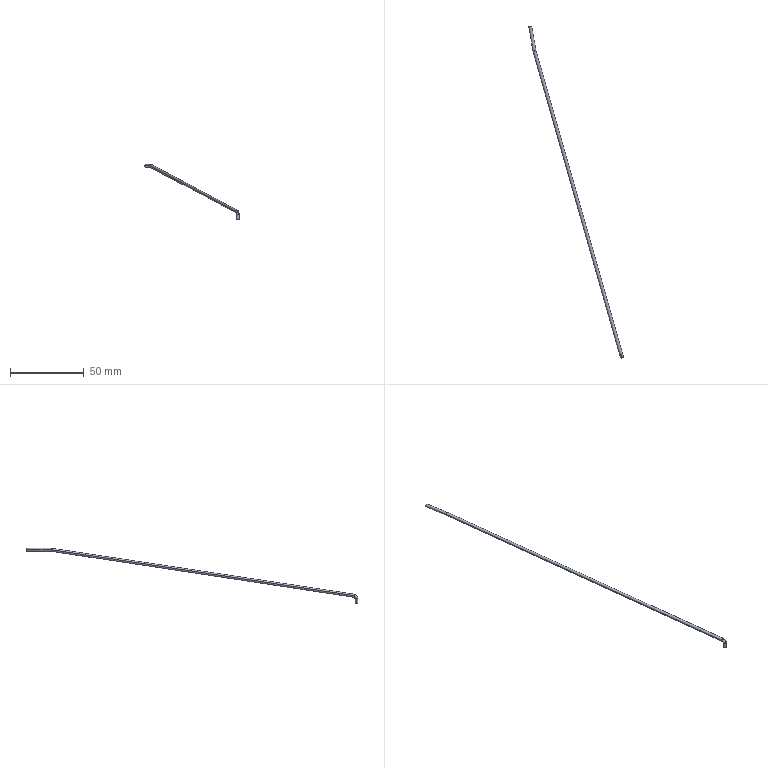Part | STEP file | rear_spoke3 | 1 solid | 10 faces | box 63.794 x 224.344 x 37.5 mm | volume 749.298 mm3 | cylinder 6 | torus 2 | plane 2 | commonest cylinder face diameters 2 x6
STEP:
#1=CARTESIAN_POINT('',(0.,0.,0.));
#2=DIRECTION('',(0.,0.,1.));
#3=DIRECTION('',(1.,0.,0.));
#4=AXIS2_PLACEMENT_3D('',#1,#2,#3);
#5=CARTESIAN_POINT('',(19.506,20.506,0.4406));
#6=VERTEX_POINT('',#5);
#7=CARTESIAN_POINT('',(20.781,19.545,0.4406));
#8=VERTEX_POINT('',#7);
#9=CARTESIAN_POINT('',(20.506,20.506,0.4406));
#10=DIRECTION('',(0.,0.,1.));
#11=DIRECTION('',(1.,0.,0.));
#12=AXIS2_PLACEMENT_3D('',#9,#10,#11);
#13=CIRCLE('',#12,1.);
#14=CARTESIAN_POINT('',(19.957,22.429,0.4406));
#15=DIRECTION('',(-0.9615,-0.2746,0.));
#16=DIRECTION('',(0.2746,-0.9615,0.));
#17=AXIS2_PLACEMENT_3D('',#14,#15,#16);
#18=TOROIDAL_SURFACE('',#17,2.,1.);
#19=CARTESIAN_POINT('',(0.,1.849));
#20=CARTESIAN_POINT('',(0.,1.821));
#21=CARTESIAN_POINT('',(0.,1.765));
#22=CARTESIAN_POINT('',(0.,1.681));
#23=CARTESIAN_POINT('',(0.,1.597));
#24=CARTESIAN_POINT('',(0.,1.513));
#25=CARTESIAN_POINT('',(0.,1.429));
#26=CARTESIAN_POINT('',(0.,1.345));
#27=CARTESIAN_POINT('',(0.,1.261));
#28=CARTESIAN_POINT('',(0.,1.177));
#29=CARTESIAN_POINT('',(0.,1.093));
#30=CARTESIAN_POINT('',(0.,1.009));
#31=CARTESIAN_POINT('',(0.,0.9245));
#32=CARTESIAN_POINT('',(0.,0.8405));
#33=CARTESIAN_POINT('',(0.,0.7564));
#34=CARTESIAN_POINT('',(0.,0.6724));
#35=CARTESIAN_POINT('',(0.,0.5883));
#36=CARTESIAN_POINT('',(0.,0.5043));
#37=CARTESIAN_POINT('',(0.,0.4202));
#38=CARTESIAN_POINT('',(0.,0.3362));
#39=CARTESIAN_POINT('',(0.,0.2521));
#40=CARTESIAN_POINT('',(0.,0.1681));
#41=CARTESIAN_POINT('',(0.,0.08405));
#42=CARTESIAN_POINT('',(0.,0.02802));
#43=CARTESIAN_POINT('',(0.,0.));
#44=B_SPLINE_CURVE_WITH_KNOTS('',3,(#19,#20,#21,#22,#23,#24,#25,#26,#27,#28,#29,#30,#31,#32,#33,#34,#35,#36,#37,#38,#39,#40,#41,#42,#43),.UNSPECIFIED.,.F.,.F.,(4,1,1,1,1,1,1,1,1,1,1,1,1,1,1,1,1,1,1,1,1,1,4),(3.142,3.226,3.31,3.394,3.478,3.562,3.646,3.73,3.814,3.898,3.982,4.066,4.15,4.234,4.318,4.402,4.486,4.57,4.654,4.738,4.823,4.907,4.991),.QUASI_UNIFORM_KNOTS.);
#45=(GEOMETRIC_REPRESENTATION_CONTEXT(2)PARAMETRIC_REPRESENTATION_CONTEXT()REPRESENTATION_CONTEXT('',''));
#46=DEFINITIONAL_REPRESENTATION('',(#44),#45);
#47=PCURVE('',#18,#46);
#48=CARTESIAN_POINT('',(20.506,20.506,-3.));
#49=DIRECTION('',(0.,0.,1.));
#50=DIRECTION('',(1.,0.,0.));
#51=AXIS2_PLACEMENT_3D('',#48,#49,#50);
#52=CYLINDRICAL_SURFACE('',#51,1.);
#53=CARTESIAN_POINT('',(0.,3.441));
#54=DIRECTION('',(1.,0.));
#55=VECTOR('',#54,1.);
#56=LINE('',#53,#55);
#57=(GEOMETRIC_REPRESENTATION_CONTEXT(2)PARAMETRIC_REPRESENTATION_CONTEXT()REPRESENTATION_CONTEXT('',''));
#58=DEFINITIONAL_REPRESENTATION('',(#56),#57);
#59=PCURVE('',#52,#58);
#60=SURFACE_CURVE('',#13,(#47,#59),.PCURVE_S1.);
#61=EDGE_CURVE('',#6,#8,#60,.T.);
#62=ORIENTED_EDGE('',*,*,#61,.T.);
#63=CARTESIAN_POINT('',(20.076,22.013,3.409));
#64=VERTEX_POINT('',#63);
#65=CARTESIAN_POINT('',(19.957,22.429,0.4406));
#66=DIRECTION('',(-0.9615,-0.2746,0.));
#67=DIRECTION('',(0.2746,-0.9615,0.));
#68=AXIS2_PLACEMENT_3D('',#65,#66,#67);
#69=CIRCLE('',#68,3.);
#70=CARTESIAN_POINT('',(0.,0.));
#71=DIRECTION('',(1.,0.));
#72=VECTOR('',#71,1.);
#73=LINE('',#70,#72);
#74=(GEOMETRIC_REPRESENTATION_CONTEXT(2)PARAMETRIC_REPRESENTATION_CONTEXT()REPRESENTATION_CONTEXT('',''));
#75=DEFINITIONAL_REPRESENTATION('',(#73),#74);
#76=PCURVE('',#18,#75);
#77=CARTESIAN_POINT('',(19.957,22.429,0.4406));
#78=DIRECTION('',(-0.9615,-0.2746,0.));
#79=DIRECTION('',(0.2746,-0.9615,0.));
#80=AXIS2_PLACEMENT_3D('',#77,#78,#79);
#81=TOROIDAL_SURFACE('',#80,2.,1.);
#82=CARTESIAN_POINT('',(0.,6.283));
#83=DIRECTION('',(1.,0.));
#84=VECTOR('',#83,1.);
#85=LINE('',#82,#84);
#86=(GEOMETRIC_REPRESENTATION_CONTEXT(2)PARAMETRIC_REPRESENTATION_CONTEXT()REPRESENTATION_CONTEXT('',''));
#87=DEFINITIONAL_REPRESENTATION('',(#85),#86);
#88=PCURVE('',#81,#87);
#89=SURFACE_CURVE('',#69,(#76,#88),.PCURVE_S1.);
#90=EDGE_CURVE('',#8,#64,#89,.T.);
#91=ORIENTED_EDGE('',*,*,#90,.T.);
#92=CARTESIAN_POINT('',(19.075,21.877,2.42));
#93=VERTEX_POINT('',#92);
#94=CARTESIAN_POINT('',(20.036,22.152,2.42));
#95=DIRECTION('',(-0.2718,0.9515,0.1444));
#96=DIRECTION('',(0.9355,0.226,0.2718));
#97=AXIS2_PLACEMENT_3D('',#94,#95,#96);
#98=CIRCLE('',#97,1.);
#99=CARTESIAN_POINT('',(1.426,4.991));
#100=DIRECTION('',(0.,-1.));
#101=VECTOR('',#100,1.);
#102=LINE('',#99,#101);
#103=(GEOMETRIC_REPRESENTATION_CONTEXT(2)PARAMETRIC_REPRESENTATION_CONTEXT()REPRESENTATION_CONTEXT('',''));
#104=DEFINITIONAL_REPRESENTATION('',(#102),#103);
#105=PCURVE('',#18,#104);
#106=CARTESIAN_POINT('',(20.036,22.152,2.42));
#107=DIRECTION('',(-0.2718,0.9515,0.1444));
#108=DIRECTION('',(-0.9615,-0.2746,0.));
#109=AXIS2_PLACEMENT_3D('',#106,#107,#108);
#110=CYLINDRICAL_SURFACE('',#109,1.);
#111=CARTESIAN_POINT('',(-3.42,0.));
#112=DIRECTION('',(1.,0.));
#113=VECTOR('',#112,1.);
#114=LINE('',#111,#113);
#115=(GEOMETRIC_REPRESENTATION_CONTEXT(2)PARAMETRIC_REPRESENTATION_CONTEXT()REPRESENTATION_CONTEXT('',''));
#116=DEFINITIONAL_REPRESENTATION('',(#114),#115);
#117=PCURVE('',#110,#116);
#118=SURFACE_CURVE('',#98,(#105,#117),.PCURVE_S1.);
#119=EDGE_CURVE('',#93,#64,#118,.T.);
#120=ORIENTED_EDGE('',*,*,#119,.F.);
#121=CARTESIAN_POINT('',(19.996,22.29,1.43));
#122=VERTEX_POINT('',#121);
#123=CARTESIAN_POINT('',(20.036,22.152,2.42));
#124=DIRECTION('',(-0.2718,0.9515,0.1444));
#125=DIRECTION('',(0.9355,0.226,0.2718));
#126=AXIS2_PLACEMENT_3D('',#123,#124,#125);
#127=CIRCLE('',#126,1.);
#128=CARTESIAN_POINT('',(1.426,4.991));
#129=DIRECTION('',(0.,-1.));
#130=VECTOR('',#129,1.);
#131=LINE('',#128,#130);
#132=(GEOMETRIC_REPRESENTATION_CONTEXT(2)PARAMETRIC_REPRESENTATION_CONTEXT()REPRESENTATION_CONTEXT('',''));
#133=DEFINITIONAL_REPRESENTATION('',(#131),#132);
#134=PCURVE('',#18,#133);
#135=CARTESIAN_POINT('',(20.036,22.152,2.42));
#136=DIRECTION('',(-0.2718,0.9515,0.1444));
#137=DIRECTION('',(-0.9615,-0.2746,0.));
#138=AXIS2_PLACEMENT_3D('',#135,#136,#137);
#139=CYLINDRICAL_SURFACE('',#138,1.);
#140=CARTESIAN_POINT('',(2.863,0.));
#141=DIRECTION('',(1.,0.));
#142=VECTOR('',#141,1.);
#143=LINE('',#140,#142);
#144=(GEOMETRIC_REPRESENTATION_CONTEXT(2)PARAMETRIC_REPRESENTATION_CONTEXT()REPRESENTATION_CONTEXT('',''));
#145=DEFINITIONAL_REPRESENTATION('',(#143),#144);
#146=PCURVE('',#139,#145);
#147=SURFACE_CURVE('',#127,(#134,#146),.PCURVE_S1.);
#148=EDGE_CURVE('',#122,#93,#147,.T.);
#149=ORIENTED_EDGE('',*,*,#148,.F.);
#150=CARTESIAN_POINT('',(20.231,21.468,0.4406));
#151=VERTEX_POINT('',#150);
#152=CARTESIAN_POINT('',(19.957,22.429,0.4406));
#153=DIRECTION('',(-0.9615,-0.2746,0.));
#154=DIRECTION('',(0.2746,-0.9615,0.));
#155=AXIS2_PLACEMENT_3D('',#152,#153,#154);
#156=CIRCLE('',#155,1.);
#157=CARTESIAN_POINT('',(0.,3.142));
#158=DIRECTION('',(1.,0.));
#159=VECTOR('',#158,1.);
#160=LINE('',#157,#159);
#161=(GEOMETRIC_REPRESENTATION_CONTEXT(2)PARAMETRIC_REPRESENTATION_CONTEXT()REPRESENTATION_CONTEXT('',''));
#162=DEFINITIONAL_REPRESENTATION('',(#160),#161);
#163=PCURVE('',#18,#162);
#164=CARTESIAN_POINT('',(0.,3.142));
#165=DIRECTION('',(1.,0.));
#166=VECTOR('',#165,1.);
#167=LINE('',#164,#166);
#168=(GEOMETRIC_REPRESENTATION_CONTEXT(2)PARAMETRIC_REPRESENTATION_CONTEXT()REPRESENTATION_CONTEXT('',''));
#169=DEFINITIONAL_REPRESENTATION('',(#167),#168);
#170=PCURVE('',#81,#169);
#171=SURFACE_CURVE('',#156,(#163,#170),.PCURVE_S1.);
#172=EDGE_CURVE('',#151,#122,#171,.T.);
#173=ORIENTED_EDGE('',*,*,#172,.F.);
#174=CARTESIAN_POINT('',(20.506,20.506,0.4406));
#175=DIRECTION('',(0.,0.,1.));
#176=DIRECTION('',(1.,0.,0.));
#177=AXIS2_PLACEMENT_3D('',#174,#175,#176);
#178=CIRCLE('',#177,1.);
#179=CARTESIAN_POINT('',(0.,4.991));
#180=DIRECTION('',(0.,-1.));
#181=VECTOR('',#180,1.);
#182=LINE('',#179,#181);
#183=(GEOMETRIC_REPRESENTATION_CONTEXT(2)PARAMETRIC_REPRESENTATION_CONTEXT()REPRESENTATION_CONTEXT('',''));
#184=DEFINITIONAL_REPRESENTATION('',(#182),#183);
#185=PCURVE('',#18,#184);
#186=CARTESIAN_POINT('',(20.506,20.506,-3.));
#187=DIRECTION('',(0.,0.,1.));
#188=DIRECTION('',(1.,0.,0.));
#189=AXIS2_PLACEMENT_3D('',#186,#187,#188);
#190=CYLINDRICAL_SURFACE('',#189,1.);
#191=CARTESIAN_POINT('',(0.,3.441));
#192=DIRECTION('',(1.,0.));
#193=VECTOR('',#192,1.);
#194=LINE('',#191,#193);
#195=(GEOMETRIC_REPRESENTATION_CONTEXT(2)PARAMETRIC_REPRESENTATION_CONTEXT()REPRESENTATION_CONTEXT('',''));
#196=DEFINITIONAL_REPRESENTATION('',(#194),#195);
#197=PCURVE('',#190,#196);
#198=SURFACE_CURVE('',#178,(#185,#197),.PCURVE_S1.);
#199=EDGE_CURVE('',#151,#6,#198,.T.);
#200=ORIENTED_EDGE('',*,*,#199,.T.);
#201=EDGE_LOOP('',(#62,#91,#120,#149,#173,#200));
#202=FACE_BOUND('',#201,.T.);
#203=ADVANCED_FACE('',(#202),#18,.T.);
#204=ORIENTED_EDGE('',*,*,#119,.T.);
#205=CARTESIAN_POINT('',(20.998,22.426,2.42));
#206=VERTEX_POINT('',#205);
#207=CARTESIAN_POINT('',(20.036,22.152,2.42));
#208=DIRECTION('',(-0.2718,0.9515,0.1444));
#209=DIRECTION('',(0.9355,0.226,0.2718));
#210=AXIS2_PLACEMENT_3D('',#207,#208,#209);
#211=CIRCLE('',#210,1.);
#212=CARTESIAN_POINT('',(-3.42,0.));
#213=DIRECTION('',(1.,0.));
#214=VECTOR('',#213,1.);
#215=LINE('',#212,#214);
#216=(GEOMETRIC_REPRESENTATION_CONTEXT(2)PARAMETRIC_REPRESENTATION_CONTEXT()REPRESENTATION_CONTEXT('',''));
#217=DEFINITIONAL_REPRESENTATION('',(#215),#216);
#218=PCURVE('',#110,#217);
#219=CARTESIAN_POINT('',(1.426,11.274));
#220=DIRECTION('',(0.,-1.));
#221=VECTOR('',#220,1.);
#222=LINE('',#219,#221);
#223=(GEOMETRIC_REPRESENTATION_CONTEXT(2)PARAMETRIC_REPRESENTATION_CONTEXT()REPRESENTATION_CONTEXT('',''));
#224=DEFINITIONAL_REPRESENTATION('',(#222),#223);
#225=PCURVE('',#81,#224);
#226=SURFACE_CURVE('',#211,(#218,#225),.PCURVE_S1.);
#227=EDGE_CURVE('',#64,#206,#226,.T.);
#228=ORIENTED_EDGE('',*,*,#227,.T.);
#229=CARTESIAN_POINT('',(-37.497,227.218,33.492));
#230=VERTEX_POINT('',#229);
#231=CARTESIAN_POINT('',(20.998,22.426,2.42));
#232=DIRECTION('',(-0.2718,0.9515,0.1444));
#233=VECTOR('',#232,1.);
#234=LINE('',#231,#233);
#235=CARTESIAN_POINT('',(3.142,0.));
#236=DIRECTION('',(0.,1.));
#237=VECTOR('',#236,1.);
#238=LINE('',#235,#237);
#239=(GEOMETRIC_REPRESENTATION_CONTEXT(2)PARAMETRIC_REPRESENTATION_CONTEXT()REPRESENTATION_CONTEXT('',''));
#240=DEFINITIONAL_REPRESENTATION('',(#238),#239);
#241=PCURVE('',#110,#240);
#242=CARTESIAN_POINT('',(3.142,0.));
#243=DIRECTION('',(0.,1.));
#244=VECTOR('',#243,1.);
#245=LINE('',#242,#244);
#246=(GEOMETRIC_REPRESENTATION_CONTEXT(2)PARAMETRIC_REPRESENTATION_CONTEXT()REPRESENTATION_CONTEXT('',''));
#247=DEFINITIONAL_REPRESENTATION('',(#245),#246);
#248=PCURVE('',#139,#247);
#249=SURFACE_CURVE('',#234,(#241,#248),.PCURVE_S1.);
#250=EDGE_CURVE('',#206,#230,#249,.T.);
#251=ORIENTED_EDGE('',*,*,#250,.T.);
#252=CARTESIAN_POINT('',(-37.497,227.218,33.5));
#253=VERTEX_POINT('',#252);
#254=CARTESIAN_POINT('',(-37.497,227.218,33.492));
#255=CARTESIAN_POINT('',(-37.497,227.218,33.495));
#256=CARTESIAN_POINT('',(-37.497,227.218,33.497));
#257=CARTESIAN_POINT('',(-37.497,227.218,33.5));
#258=(BOUNDED_CURVE()B_SPLINE_CURVE(3,(#254,#255,#256,#257),.UNSPECIFIED.,.F.,.F.)B_SPLINE_CURVE_WITH_KNOTS((4,4),(4.058,4.066),.PIECEWISE_BEZIER_KNOTS.)CURVE()GEOMETRIC_REPRESENTATION_ITEM()RATIONAL_B_SPLINE_CURVE((1.,1.,1.,1.))REPRESENTATION_ITEM(''));
#259=CARTESIAN_POINT('',(3.142,215.237));
#260=CARTESIAN_POINT('',(3.134,215.238));
#261=B_SPLINE_CURVE_WITH_KNOTS('',1,(#259,#260),.UNSPECIFIED.,.F.,.F.,(2,2),(4.058,4.066),.PIECEWISE_BEZIER_KNOTS.);
#262=(GEOMETRIC_REPRESENTATION_CONTEXT(2)PARAMETRIC_REPRESENTATION_CONTEXT()REPRESENTATION_CONTEXT('',''));
#263=DEFINITIONAL_REPRESENTATION('',(#261),#262);
#264=PCURVE('',#110,#263);
#265=CARTESIAN_POINT('',(-38.42,226.678,33.5));
#266=DIRECTION('',(-0.1671,0.9859,0.));
#267=DIRECTION('',(-0.9859,-0.1671,0.));
#268=AXIS2_PLACEMENT_3D('',#265,#266,#267);
#269=CYLINDRICAL_SURFACE('',#268,1.);
#270=CARTESIAN_POINT('',(3.15,0.3789));
#271=CARTESIAN_POINT('',(3.142,0.3784));
#272=B_SPLINE_CURVE_WITH_KNOTS('',1,(#270,#271),.UNSPECIFIED.,.F.,.F.,(2,2),(4.058,4.066),.PIECEWISE_BEZIER_KNOTS.);
#273=(GEOMETRIC_REPRESENTATION_CONTEXT(2)PARAMETRIC_REPRESENTATION_CONTEXT()REPRESENTATION_CONTEXT('',''));
#274=DEFINITIONAL_REPRESENTATION('',(#272),#273);
#275=PCURVE('',#269,#274);
#276=SURFACE_CURVE('',#258,(#264,#275),.PCURVE_S1.);
#277=EDGE_CURVE('',#230,#253,#276,.T.);
#278=ORIENTED_EDGE('',*,*,#277,.T.);
#279=CARTESIAN_POINT('',(-39.45,226.775,33.508));
#280=VERTEX_POINT('',#279);
#281=CARTESIAN_POINT('',(-37.497,227.218,33.5));
#282=CARTESIAN_POINT('',(-37.473,227.075,35.484));
#283=CARTESIAN_POINT('',(-39.411,226.636,35.492));
#284=CARTESIAN_POINT('',(-39.45,226.775,33.508));
#285=(BOUNDED_CURVE()B_SPLINE_CURVE(3,(#281,#282,#283,#284),.UNSPECIFIED.,.F.,.F.)B_SPLINE_CURVE_WITH_KNOTS((4,4),(4.066,7.199),.PIECEWISE_BEZIER_KNOTS.)CURVE()GEOMETRIC_REPRESENTATION_ITEM()RATIONAL_B_SPLINE_CURVE((1.,0.336,0.336,1.))REPRESENTATION_ITEM(''));
#286=CARTESIAN_POINT('',(3.134,215.238));
#287=CARTESIAN_POINT('',(3.103,215.24));
#288=CARTESIAN_POINT('',(3.04,215.244));
#289=CARTESIAN_POINT('',(2.936,215.253));
#290=CARTESIAN_POINT('',(2.822,215.262));
#291=CARTESIAN_POINT('',(2.698,215.273));
#292=CARTESIAN_POINT('',(2.564,215.285));
#293=CARTESIAN_POINT('',(2.419,215.299));
#294=CARTESIAN_POINT('',(2.263,215.313));
#295=CARTESIAN_POINT('',(2.099,215.327));
#296=CARTESIAN_POINT('',(1.926,215.341));
#297=CARTESIAN_POINT('',(1.748,215.354));
#298=CARTESIAN_POINT('',(1.567,215.365));
#299=CARTESIAN_POINT('',(1.386,215.374));
#300=CARTESIAN_POINT('',(1.208,215.38));
#301=CARTESIAN_POINT('',(1.035,215.383));
#302=CARTESIAN_POINT('',(0.8703,215.384));
#303=CARTESIAN_POINT('',(0.7148,215.382));
#304=CARTESIAN_POINT('',(0.5697,215.378));
#305=CARTESIAN_POINT('',(0.4352,215.373));
#306=CARTESIAN_POINT('',(0.3113,215.368));
#307=CARTESIAN_POINT('',(0.1976,215.361));
#308=CARTESIAN_POINT('',(0.09365,215.355));
#309=CARTESIAN_POINT('',(0.0303,215.35));
#310=CARTESIAN_POINT('',(0.,215.348));
#311=B_SPLINE_CURVE_WITH_KNOTS('',3,(#286,#287,#288,#289,#290,#291,#292,#293,#294,#295,#296,#297,#298,#299,#300,#301,#302,#303,#304,#305,#306,#307,#308,#309,#310),.UNSPECIFIED.,.F.,.F.,(4,1,1,1,1,1,1,1,1,1,1,1,1,1,1,1,1,1,1,1,1,1,4),(4.066,4.208,4.351,4.493,4.636,4.778,4.921,5.063,5.205,5.348,5.49,5.633,5.775,5.918,6.06,6.202,6.345,6.487,6.63,6.772,6.915,7.057,7.199),.QUASI_UNIFORM_KNOTS.);
#312=(GEOMETRIC_REPRESENTATION_CONTEXT(2)PARAMETRIC_REPRESENTATION_CONTEXT()REPRESENTATION_CONTEXT('',''));
#313=DEFINITIONAL_REPRESENTATION('',(#311),#312);
#314=PCURVE('',#110,#313);
#315=CARTESIAN_POINT('',(-38.42,226.678,33.5));
#316=DIRECTION('',(-0.1671,0.9859,0.));
#317=DIRECTION('',(-0.9859,-0.1671,0.));
#318=AXIS2_PLACEMENT_3D('',#315,#316,#317);
#319=CYLINDRICAL_SURFACE('',#318,1.);
#320=CARTESIAN_POINT('',(3.142,0.3784));
#321=CARTESIAN_POINT('',(3.111,0.3761));
#322=CARTESIAN_POINT('',(3.048,0.3714));
#323=CARTESIAN_POINT('',(2.944,0.3631));
#324=CARTESIAN_POINT('',(2.83,0.3535));
#325=CARTESIAN_POINT('',(2.706,0.3426));
#326=CARTESIAN_POINT('',(2.572,0.3304));
#327=CARTESIAN_POINT('',(2.427,0.3172));
#328=CARTESIAN_POINT('',(2.271,0.3031));
#329=CARTESIAN_POINT('',(2.107,0.2887));
#330=CARTESIAN_POINT('',(1.934,0.2747));
#331=CARTESIAN_POINT('',(1.756,0.2617));
#332=CARTESIAN_POINT('',(1.575,0.2505));
#333=CARTESIAN_POINT('',(1.394,0.2417));
#334=CARTESIAN_POINT('',(1.216,0.2356));
#335=CARTESIAN_POINT('',(1.043,0.2325));
#336=CARTESIAN_POINT('',(0.8783,0.2319));
#337=CARTESIAN_POINT('',(0.7229,0.2337));
#338=CARTESIAN_POINT('',(0.5777,0.2374));
#339=CARTESIAN_POINT('',(0.4432,0.2424));
#340=CARTESIAN_POINT('',(0.3193,0.2482));
#341=CARTESIAN_POINT('',(0.2057,0.2547));
#342=CARTESIAN_POINT('',(0.1017,0.2613));
#343=CARTESIAN_POINT('',(0.03831,0.2657));
#344=CARTESIAN_POINT('',(0.008014,0.2679));
#345=B_SPLINE_CURVE_WITH_KNOTS('',3,(#320,#321,#322,#323,#324,#325,#326,#327,#328,#329,#330,#331,#332,#333,#334,#335,#336,#337,#338,#339,#340,#341,#342,#343,#344),.UNSPECIFIED.,.F.,.F.,(4,1,1,1,1,1,1,1,1,1,1,1,1,1,1,1,1,1,1,1,1,1,4),(4.066,4.208,4.351,4.493,4.636,4.778,4.921,5.063,5.205,5.348,5.49,5.633,5.775,5.918,6.06,6.202,6.345,6.487,6.63,6.772,6.915,7.057,7.199),.QUASI_UNIFORM_KNOTS.);
#346=(GEOMETRIC_REPRESENTATION_CONTEXT(2)PARAMETRIC_REPRESENTATION_CONTEXT()REPRESENTATION_CONTEXT('',''));
#347=DEFINITIONAL_REPRESENTATION('',(#345),#346);
#348=PCURVE('',#319,#347);
#349=SURFACE_CURVE('',#285,(#314,#348),.PCURVE_S1.);
#350=EDGE_CURVE('',#253,#280,#349,.T.);
#351=ORIENTED_EDGE('',*,*,#350,.T.);
#352=CARTESIAN_POINT('',(19.075,21.877,2.42));
#353=DIRECTION('',(-0.2718,0.9515,0.1444));
#354=VECTOR('',#353,1.);
#355=LINE('',#352,#354);
#356=CARTESIAN_POINT('',(0.,0.));
#357=DIRECTION('',(0.,1.));
#358=VECTOR('',#357,1.);
#359=LINE('',#356,#358);
#360=(GEOMETRIC_REPRESENTATION_CONTEXT(2)PARAMETRIC_REPRESENTATION_CONTEXT()REPRESENTATION_CONTEXT('',''));
#361=DEFINITIONAL_REPRESENTATION('',(#359),#360);
#362=PCURVE('',#110,#361);
#363=CARTESIAN_POINT('',(6.283,0.));
#364=DIRECTION('',(0.,1.));
#365=VECTOR('',#364,1.);
#366=LINE('',#363,#365);
#367=(GEOMETRIC_REPRESENTATION_CONTEXT(2)PARAMETRIC_REPRESENTATION_CONTEXT()REPRESENTATION_CONTEXT('',''));
#368=DEFINITIONAL_REPRESENTATION('',(#366),#367);
#369=PCURVE('',#139,#368);
#370=SURFACE_CURVE('',#355,(#362,#369),.PCURVE_S1.);
#371=EDGE_CURVE('',#93,#280,#370,.T.);
#372=ORIENTED_EDGE('',*,*,#371,.F.);
#373=EDGE_LOOP('',(#204,#228,#251,#278,#351,#372));
#374=FACE_BOUND('',#373,.T.);
#375=ADVANCED_FACE('',(#374),#110,.T.);
#376=CARTESIAN_POINT('',(21.506,20.506,-3.));
#377=VERTEX_POINT('',#376);
#378=CARTESIAN_POINT('',(19.506,20.506,-3.));
#379=VERTEX_POINT('',#378);
#380=CARTESIAN_POINT('',(20.506,20.506,-3.));
#381=DIRECTION('',(0.,0.,1.));
#382=DIRECTION('',(1.,0.,0.));
#383=AXIS2_PLACEMENT_3D('',#380,#381,#382);
#384=CIRCLE('',#383,1.);
#385=CARTESIAN_POINT('',(0.,0.));
#386=DIRECTION('',(1.,0.));
#387=VECTOR('',#386,1.);
#388=LINE('',#385,#387);
#389=(GEOMETRIC_REPRESENTATION_CONTEXT(2)PARAMETRIC_REPRESENTATION_CONTEXT()REPRESENTATION_CONTEXT('',''));
#390=DEFINITIONAL_REPRESENTATION('',(#388),#389);
#391=PCURVE('',#190,#390);
#392=CARTESIAN_POINT('',(20.506,20.506,-3.));
#393=DIRECTION('',(0.,0.,1.));
#394=DIRECTION('',(1.,0.,0.));
#395=AXIS2_PLACEMENT_3D('',#392,#393,#394);
#396=PLANE('',#395);
#397=CARTESIAN_POINT('',(0.,0.));
#398=DIRECTION('',(1.,0.));
#399=AXIS2_PLACEMENT_2D('',#397,#398);
#400=CIRCLE('',#399,1.);
#401=(GEOMETRIC_REPRESENTATION_CONTEXT(2)PARAMETRIC_REPRESENTATION_CONTEXT()REPRESENTATION_CONTEXT('',''));
#402=DEFINITIONAL_REPRESENTATION('',(#400),#401);
#403=PCURVE('',#396,#402);
#404=SURFACE_CURVE('',#384,(#391,#403),.PCURVE_S1.);
#405=EDGE_CURVE('',#377,#379,#404,.T.);
#406=ORIENTED_EDGE('',*,*,#405,.T.);
#407=CARTESIAN_POINT('',(19.506,20.506,-3.));
#408=DIRECTION('',(0.,0.,1.));
#409=VECTOR('',#408,1.);
#410=LINE('',#407,#409);
#411=CARTESIAN_POINT('',(3.142,0.));
#412=DIRECTION('',(0.,1.));
#413=VECTOR('',#412,1.);
#414=LINE('',#411,#413);
#415=(GEOMETRIC_REPRESENTATION_CONTEXT(2)PARAMETRIC_REPRESENTATION_CONTEXT()REPRESENTATION_CONTEXT('',''));
#416=DEFINITIONAL_REPRESENTATION('',(#414),#415);
#417=PCURVE('',#190,#416);
#418=CARTESIAN_POINT('',(3.142,0.));
#419=DIRECTION('',(0.,1.));
#420=VECTOR('',#419,1.);
#421=LINE('',#418,#420);
#422=(GEOMETRIC_REPRESENTATION_CONTEXT(2)PARAMETRIC_REPRESENTATION_CONTEXT()REPRESENTATION_CONTEXT('',''));
#423=DEFINITIONAL_REPRESENTATION('',(#421),#422);
#424=PCURVE('',#52,#423);
#425=SURFACE_CURVE('',#410,(#417,#424),.PCURVE_S1.);
#426=EDGE_CURVE('',#379,#6,#425,.T.);
#427=ORIENTED_EDGE('',*,*,#426,.T.);
#428=ORIENTED_EDGE('',*,*,#199,.F.);
#429=CARTESIAN_POINT('',(21.506,20.506,0.4406));
#430=VERTEX_POINT('',#429);
#431=CARTESIAN_POINT('',(20.506,20.506,0.4406));
#432=DIRECTION('',(0.,0.,1.));
#433=DIRECTION('',(1.,0.,0.));
#434=AXIS2_PLACEMENT_3D('',#431,#432,#433);
#435=CIRCLE('',#434,1.);
#436=CARTESIAN_POINT('',(0.,3.441));
#437=DIRECTION('',(1.,0.));
#438=VECTOR('',#437,1.);
#439=LINE('',#436,#438);
#440=(GEOMETRIC_REPRESENTATION_CONTEXT(2)PARAMETRIC_REPRESENTATION_CONTEXT()REPRESENTATION_CONTEXT('',''));
#441=DEFINITIONAL_REPRESENTATION('',(#439),#440);
#442=PCURVE('',#190,#441);
#443=CARTESIAN_POINT('',(0.,4.991));
#444=DIRECTION('',(0.,-1.));
#445=VECTOR('',#444,1.);
#446=LINE('',#443,#445);
#447=(GEOMETRIC_REPRESENTATION_CONTEXT(2)PARAMETRIC_REPRESENTATION_CONTEXT()REPRESENTATION_CONTEXT('',''));
#448=DEFINITIONAL_REPRESENTATION('',(#446),#447);
#449=PCURVE('',#81,#448);
#450=SURFACE_CURVE('',#435,(#442,#449),.PCURVE_S1.);
#451=EDGE_CURVE('',#430,#151,#450,.T.);
#452=ORIENTED_EDGE('',*,*,#451,.F.);
#453=CARTESIAN_POINT('',(21.506,20.506,-3.));
#454=DIRECTION('',(0.,0.,1.));
#455=VECTOR('',#454,1.);
#456=LINE('',#453,#455);
#457=CARTESIAN_POINT('',(0.,0.));
#458=DIRECTION('',(0.,1.));
#459=VECTOR('',#458,1.);
#460=LINE('',#457,#459);
#461=(GEOMETRIC_REPRESENTATION_CONTEXT(2)PARAMETRIC_REPRESENTATION_CONTEXT()REPRESENTATION_CONTEXT('',''));
#462=DEFINITIONAL_REPRESENTATION('',(#460),#461);
#463=PCURVE('',#190,#462);
#464=CARTESIAN_POINT('',(6.283,0.));
#465=DIRECTION('',(0.,1.));
#466=VECTOR('',#465,1.);
#467=LINE('',#464,#466);
#468=(GEOMETRIC_REPRESENTATION_CONTEXT(2)PARAMETRIC_REPRESENTATION_CONTEXT()REPRESENTATION_CONTEXT('',''));
#469=DEFINITIONAL_REPRESENTATION('',(#467),#468);
#470=PCURVE('',#52,#469);
#471=SURFACE_CURVE('',#456,(#463,#470),.PCURVE_S1.);
#472=EDGE_CURVE('',#377,#430,#471,.T.);
#473=ORIENTED_EDGE('',*,*,#472,.F.);
#474=EDGE_LOOP('',(#406,#427,#428,#452,#473));
#475=FACE_BOUND('',#474,.T.);
#476=ADVANCED_FACE('',(#475),#190,.T.);
#477=ORIENTED_EDGE('',*,*,#350,.F.);
#478=CARTESIAN_POINT('',(-40.316,243.85,33.5));
#479=VERTEX_POINT('',#478);
#480=CARTESIAN_POINT('',(-37.434,226.845,33.5));
#481=DIRECTION('',(-0.1671,0.9859,0.));
#482=VECTOR('',#481,1.);
#483=LINE('',#480,#482);
#484=CARTESIAN_POINT('',(3.142,0.));
#485=DIRECTION('',(0.,1.));
#486=VECTOR('',#485,1.);
#487=LINE('',#484,#486);
#488=(GEOMETRIC_REPRESENTATION_CONTEXT(2)PARAMETRIC_REPRESENTATION_CONTEXT()REPRESENTATION_CONTEXT('',''));
#489=DEFINITIONAL_REPRESENTATION('',(#487),#488);
#490=PCURVE('',#319,#489);
#491=CARTESIAN_POINT('',(3.142,0.));
#492=DIRECTION('',(0.,1.));
#493=VECTOR('',#492,1.);
#494=LINE('',#491,#493);
#495=(GEOMETRIC_REPRESENTATION_CONTEXT(2)PARAMETRIC_REPRESENTATION_CONTEXT()REPRESENTATION_CONTEXT('',''));
#496=DEFINITIONAL_REPRESENTATION('',(#494),#495);
#497=PCURVE('',#269,#496);
#498=SURFACE_CURVE('',#483,(#490,#497),.PCURVE_S1.);
#499=EDGE_CURVE('',#253,#479,#498,.T.);
#500=ORIENTED_EDGE('',*,*,#499,.T.);
#501=CARTESIAN_POINT('',(-42.288,243.515,33.5));
#502=VERTEX_POINT('',#501);
#503=CARTESIAN_POINT('',(-41.302,243.682,33.5));
#504=DIRECTION('',(-0.1671,0.9859,0.));
#505=DIRECTION('',(0.9502,0.161,0.2669));
#506=AXIS2_PLACEMENT_3D('',#503,#504,#505);
#507=CIRCLE('',#506,1.);
#508=CARTESIAN_POINT('',(-3.412,17.247));
#509=DIRECTION('',(1.,0.));
#510=VECTOR('',#509,1.);
#511=LINE('',#508,#510);
#512=(GEOMETRIC_REPRESENTATION_CONTEXT(2)PARAMETRIC_REPRESENTATION_CONTEXT()REPRESENTATION_CONTEXT('',''));
#513=DEFINITIONAL_REPRESENTATION('',(#511),#512);
#514=PCURVE('',#319,#513);
#515=CARTESIAN_POINT('',(-41.302,243.682,33.5));
#516=DIRECTION('',(-0.1671,0.9859,0.));
#517=DIRECTION('',(0.9502,0.161,0.2669));
#518=AXIS2_PLACEMENT_3D('',#515,#516,#517);
#519=PLANE('',#518);
#520=CARTESIAN_POINT('',(0.,0.));
#521=DIRECTION('',(1.,0.));
#522=AXIS2_PLACEMENT_2D('',#520,#521);
#523=CIRCLE('',#522,1.);
#524=(GEOMETRIC_REPRESENTATION_CONTEXT(2)PARAMETRIC_REPRESENTATION_CONTEXT()REPRESENTATION_CONTEXT('',''));
#525=DEFINITIONAL_REPRESENTATION('',(#523),#524);
#526=PCURVE('',#519,#525);
#527=SURFACE_CURVE('',#507,(#514,#526),.PCURVE_S1.);
#528=EDGE_CURVE('',#502,#479,#527,.T.);
#529=ORIENTED_EDGE('',*,*,#528,.F.);
#530=CARTESIAN_POINT('',(-39.45,226.775,33.5));
#531=VERTEX_POINT('',#530);
#532=CARTESIAN_POINT('',(-39.406,226.511,33.5));
#533=DIRECTION('',(-0.1671,0.9859,0.));
#534=VECTOR('',#533,1.);
#535=LINE('',#532,#534);
#536=CARTESIAN_POINT('',(0.,0.));
#537=DIRECTION('',(0.,1.));
#538=VECTOR('',#537,1.);
#539=LINE('',#536,#538);
#540=(GEOMETRIC_REPRESENTATION_CONTEXT(2)PARAMETRIC_REPRESENTATION_CONTEXT()REPRESENTATION_CONTEXT('',''));
#541=DEFINITIONAL_REPRESENTATION('',(#539),#540);
#542=PCURVE('',#319,#541);
#543=CARTESIAN_POINT('',(6.283,0.));
#544=DIRECTION('',(0.,1.));
#545=VECTOR('',#544,1.);
#546=LINE('',#543,#545);
#547=(GEOMETRIC_REPRESENTATION_CONTEXT(2)PARAMETRIC_REPRESENTATION_CONTEXT()REPRESENTATION_CONTEXT('',''));
#548=DEFINITIONAL_REPRESENTATION('',(#546),#547);
#549=PCURVE('',#269,#548);
#550=SURFACE_CURVE('',#535,(#542,#549),.PCURVE_S1.);
#551=EDGE_CURVE('',#531,#502,#550,.T.);
#552=ORIENTED_EDGE('',*,*,#551,.F.);
#553=CARTESIAN_POINT('',(-39.45,226.775,33.508));
#554=CARTESIAN_POINT('',(-39.45,226.775,33.505));
#555=CARTESIAN_POINT('',(-39.45,226.775,33.503));
#556=CARTESIAN_POINT('',(-39.45,226.775,33.5));
#557=(BOUNDED_CURVE()B_SPLINE_CURVE(3,(#553,#554,#555,#556),.UNSPECIFIED.,.F.,.F.)B_SPLINE_CURVE_WITH_KNOTS((4,4),(0.9163,0.9243),.PIECEWISE_BEZIER_KNOTS.)CURVE()GEOMETRIC_REPRESENTATION_ITEM()RATIONAL_B_SPLINE_CURVE((1.,1.,1.,1.))REPRESENTATION_ITEM(''));
#558=CARTESIAN_POINT('',(0.008014,0.2679));
#559=CARTESIAN_POINT('',(0.,0.2685));
#560=B_SPLINE_CURVE_WITH_KNOTS('',1,(#558,#559),.UNSPECIFIED.,.F.,.F.,(2,2),(0.9163,0.9243),.PIECEWISE_BEZIER_KNOTS.);
#561=(GEOMETRIC_REPRESENTATION_CONTEXT(2)PARAMETRIC_REPRESENTATION_CONTEXT()REPRESENTATION_CONTEXT('',''));
#562=DEFINITIONAL_REPRESENTATION('',(#560),#561);
#563=PCURVE('',#319,#562);
#564=CARTESIAN_POINT('',(6.283,215.348));
#565=CARTESIAN_POINT('',(6.275,215.347));
#566=B_SPLINE_CURVE_WITH_KNOTS('',1,(#564,#565),.UNSPECIFIED.,.F.,.F.,(2,2),(0.9163,0.9243),.PIECEWISE_BEZIER_KNOTS.);
#567=(GEOMETRIC_REPRESENTATION_CONTEXT(2)PARAMETRIC_REPRESENTATION_CONTEXT()REPRESENTATION_CONTEXT('',''));
#568=DEFINITIONAL_REPRESENTATION('',(#566),#567);
#569=PCURVE('',#139,#568);
#570=SURFACE_CURVE('',#557,(#563,#569),.PCURVE_S1.);
#571=EDGE_CURVE('',#280,#531,#570,.T.);
#572=ORIENTED_EDGE('',*,*,#571,.F.);
#573=EDGE_LOOP('',(#477,#500,#529,#552,#572));
#574=FACE_BOUND('',#573,.T.);
#575=ADVANCED_FACE('',(#574),#319,.T.);
#576=ORIENTED_EDGE('',*,*,#250,.F.);
#577=CARTESIAN_POINT('',(20.036,22.152,2.42));
#578=DIRECTION('',(-0.2718,0.9515,0.1444));
#579=DIRECTION('',(0.9355,0.226,0.2718));
#580=AXIS2_PLACEMENT_3D('',#577,#578,#579);
#581=CIRCLE('',#580,1.);
#582=CARTESIAN_POINT('',(2.863,0.));
#583=DIRECTION('',(1.,0.));
#584=VECTOR('',#583,1.);
#585=LINE('',#582,#584);
#586=(GEOMETRIC_REPRESENTATION_CONTEXT(2)PARAMETRIC_REPRESENTATION_CONTEXT()REPRESENTATION_CONTEXT('',''));
#587=DEFINITIONAL_REPRESENTATION('',(#585),#586);
#588=PCURVE('',#139,#587);
#589=CARTESIAN_POINT('',(1.426,4.991));
#590=DIRECTION('',(0.,-1.));
#591=VECTOR('',#590,1.);
#592=LINE('',#589,#591);
#593=(GEOMETRIC_REPRESENTATION_CONTEXT(2)PARAMETRIC_REPRESENTATION_CONTEXT()REPRESENTATION_CONTEXT('',''));
#594=DEFINITIONAL_REPRESENTATION('',(#592),#593);
#595=PCURVE('',#81,#594);
#596=SURFACE_CURVE('',#581,(#588,#595),.PCURVE_S1.);
#597=EDGE_CURVE('',#206,#122,#596,.T.);
#598=ORIENTED_EDGE('',*,*,#597,.T.);
#599=ORIENTED_EDGE('',*,*,#148,.T.);
#600=ORIENTED_EDGE('',*,*,#371,.T.);
#601=ORIENTED_EDGE('',*,*,#571,.T.);
#602=CARTESIAN_POINT('',(-39.45,226.775,33.5));
#603=CARTESIAN_POINT('',(-39.475,226.918,31.516));
#604=CARTESIAN_POINT('',(-37.537,227.357,31.508));
#605=CARTESIAN_POINT('',(-37.497,227.218,33.492));
#606=(BOUNDED_CURVE()B_SPLINE_CURVE(3,(#602,#603,#604,#605),.UNSPECIFIED.,.F.,.F.)B_SPLINE_CURVE_WITH_KNOTS((4,4),(0.9243,4.058),.PIECEWISE_BEZIER_KNOTS.)CURVE()GEOMETRIC_REPRESENTATION_ITEM()RATIONAL_B_SPLINE_CURVE((1.,0.336,0.336,1.))REPRESENTATION_ITEM(''));
#607=CARTESIAN_POINT('',(6.275,215.347));
#608=CARTESIAN_POINT('',(6.245,215.345));
#609=CARTESIAN_POINT('',(6.182,215.34));
#610=CARTESIAN_POINT('',(6.078,215.332));
#611=CARTESIAN_POINT('',(5.964,215.322));
#612=CARTESIAN_POINT('',(5.84,215.312));
#613=CARTESIAN_POINT('',(5.705,215.299));
#614=CARTESIAN_POINT('',(5.56,215.286));
#615=CARTESIAN_POINT('',(5.405,215.272));
#616=CARTESIAN_POINT('',(5.24,215.258));
#617=CARTESIAN_POINT('',(5.068,215.244));
#618=CARTESIAN_POINT('',(4.889,215.231));
#619=CARTESIAN_POINT('',(4.708,215.219));
#620=CARTESIAN_POINT('',(4.527,215.211));
#621=CARTESIAN_POINT('',(4.349,215.205));
#622=CARTESIAN_POINT('',(4.177,215.201));
#623=CARTESIAN_POINT('',(4.012,215.201));
#624=CARTESIAN_POINT('',(3.856,215.203));
#625=CARTESIAN_POINT('',(3.711,215.206));
#626=CARTESIAN_POINT('',(3.577,215.211));
#627=CARTESIAN_POINT('',(3.453,215.217));
#628=CARTESIAN_POINT('',(3.339,215.224));
#629=CARTESIAN_POINT('',(3.235,215.23));
#630=CARTESIAN_POINT('',(3.172,215.235));
#631=CARTESIAN_POINT('',(3.142,215.237));
#632=B_SPLINE_CURVE_WITH_KNOTS('',3,(#607,#608,#609,#610,#611,#612,#613,#614,#615,#616,#617,#618,#619,#620,#621,#622,#623,#624,#625,#626,#627,#628,#629,#630,#631),.UNSPECIFIED.,.F.,.F.,(4,1,1,1,1,1,1,1,1,1,1,1,1,1,1,1,1,1,1,1,1,1,4),(0.9243,1.067,1.209,1.352,1.494,1.636,1.779,1.921,2.064,2.206,2.349,2.491,2.634,2.776,2.918,3.061,3.203,3.346,3.488,3.631,3.773,3.915,4.058),.QUASI_UNIFORM_KNOTS.);
#633=(GEOMETRIC_REPRESENTATION_CONTEXT(2)PARAMETRIC_REPRESENTATION_CONTEXT()REPRESENTATION_CONTEXT('',''));
#634=DEFINITIONAL_REPRESENTATION('',(#632),#633);
#635=PCURVE('',#139,#634);
#636=CARTESIAN_POINT('',(6.283,0.2685));
#637=CARTESIAN_POINT('',(6.253,0.2707));
#638=CARTESIAN_POINT('',(6.19,0.2755));
#639=CARTESIAN_POINT('',(6.086,0.2838));
#640=CARTESIAN_POINT('',(5.972,0.2934));
#641=CARTESIAN_POINT('',(5.848,0.3042));
#642=CARTESIAN_POINT('',(5.714,0.3164));
#643=CARTESIAN_POINT('',(5.568,0.3297));
#644=CARTESIAN_POINT('',(5.413,0.3437));
#645=CARTESIAN_POINT('',(5.248,0.3581));
#646=CARTESIAN_POINT('',(5.076,0.3722));
#647=CARTESIAN_POINT('',(4.897,0.3852));
#648=CARTESIAN_POINT('',(4.716,0.3964));
#649=CARTESIAN_POINT('',(4.535,0.4052));
#650=CARTESIAN_POINT('',(4.357,0.4112));
#651=CARTESIAN_POINT('',(4.185,0.4144));
#652=CARTESIAN_POINT('',(4.02,0.4149));
#653=CARTESIAN_POINT('',(3.864,0.4131));
#654=CARTESIAN_POINT('',(3.719,0.4095));
#655=CARTESIAN_POINT('',(3.585,0.4045));
#656=CARTESIAN_POINT('',(3.461,0.3986));
#657=CARTESIAN_POINT('',(3.347,0.3922));
#658=CARTESIAN_POINT('',(3.243,0.3856));
#659=CARTESIAN_POINT('',(3.18,0.3811));
#660=CARTESIAN_POINT('',(3.15,0.3789));
#661=B_SPLINE_CURVE_WITH_KNOTS('',3,(#636,#637,#638,#639,#640,#641,#642,#643,#644,#645,#646,#647,#648,#649,#650,#651,#652,#653,#654,#655,#656,#657,#658,#659,#660),.UNSPECIFIED.,.F.,.F.,(4,1,1,1,1,1,1,1,1,1,1,1,1,1,1,1,1,1,1,1,1,1,4),(0.9243,1.067,1.209,1.352,1.494,1.636,1.779,1.921,2.064,2.206,2.349,2.491,2.634,2.776,2.918,3.061,3.203,3.346,3.488,3.631,3.773,3.915,4.058),.QUASI_UNIFORM_KNOTS.);
#662=(GEOMETRIC_REPRESENTATION_CONTEXT(2)PARAMETRIC_REPRESENTATION_CONTEXT()REPRESENTATION_CONTEXT('',''));
#663=DEFINITIONAL_REPRESENTATION('',(#661),#662);
#664=PCURVE('',#269,#663);
#665=SURFACE_CURVE('',#606,(#635,#664),.PCURVE_S1.);
#666=EDGE_CURVE('',#531,#230,#665,.T.);
#667=ORIENTED_EDGE('',*,*,#666,.T.);
#668=EDGE_LOOP('',(#576,#598,#599,#600,#601,#667));
#669=FACE_BOUND('',#668,.T.);
#670=ADVANCED_FACE('',(#669),#139,.T.);
#671=ORIENTED_EDGE('',*,*,#90,.F.);
#672=CARTESIAN_POINT('',(20.506,20.506,0.4406));
#673=DIRECTION('',(0.,0.,1.));
#674=DIRECTION('',(1.,0.,0.));
#675=AXIS2_PLACEMENT_3D('',#672,#673,#674);
#676=CIRCLE('',#675,1.);
#677=CARTESIAN_POINT('',(0.,11.274));
#678=DIRECTION('',(0.,-1.));
#679=VECTOR('',#678,1.);
#680=LINE('',#677,#679);
#681=(GEOMETRIC_REPRESENTATION_CONTEXT(2)PARAMETRIC_REPRESENTATION_CONTEXT()REPRESENTATION_CONTEXT('',''));
#682=DEFINITIONAL_REPRESENTATION('',(#680),#681);
#683=PCURVE('',#81,#682);
#684=CARTESIAN_POINT('',(0.,3.441));
#685=DIRECTION('',(1.,0.));
#686=VECTOR('',#685,1.);
#687=LINE('',#684,#686);
#688=(GEOMETRIC_REPRESENTATION_CONTEXT(2)PARAMETRIC_REPRESENTATION_CONTEXT()REPRESENTATION_CONTEXT('',''));
#689=DEFINITIONAL_REPRESENTATION('',(#687),#688);
#690=PCURVE('',#52,#689);
#691=SURFACE_CURVE('',#676,(#683,#690),.PCURVE_S1.);
#692=EDGE_CURVE('',#8,#430,#691,.T.);
#693=ORIENTED_EDGE('',*,*,#692,.T.);
#694=ORIENTED_EDGE('',*,*,#451,.T.);
#695=ORIENTED_EDGE('',*,*,#172,.T.);
#696=ORIENTED_EDGE('',*,*,#597,.F.);
#697=ORIENTED_EDGE('',*,*,#227,.F.);
#698=EDGE_LOOP('',(#671,#693,#694,#695,#696,#697));
#699=FACE_BOUND('',#698,.T.);
#700=ADVANCED_FACE('',(#699),#81,.T.);
#701=ORIENTED_EDGE('',*,*,#426,.F.);
#702=CARTESIAN_POINT('',(20.506,20.506,-3.));
#703=DIRECTION('',(0.,0.,1.));
#704=DIRECTION('',(1.,0.,0.));
#705=AXIS2_PLACEMENT_3D('',#702,#703,#704);
#706=CIRCLE('',#705,1.);
#707=CARTESIAN_POINT('',(0.,0.));
#708=DIRECTION('',(1.,0.));
#709=VECTOR('',#708,1.);
#710=LINE('',#707,#709);
#711=(GEOMETRIC_REPRESENTATION_CONTEXT(2)PARAMETRIC_REPRESENTATION_CONTEXT()REPRESENTATION_CONTEXT('',''));
#712=DEFINITIONAL_REPRESENTATION('',(#710),#711);
#713=PCURVE('',#52,#712);
#714=CARTESIAN_POINT('',(0.,0.));
#715=DIRECTION('',(1.,0.));
#716=AXIS2_PLACEMENT_2D('',#714,#715);
#717=CIRCLE('',#716,1.);
#718=(GEOMETRIC_REPRESENTATION_CONTEXT(2)PARAMETRIC_REPRESENTATION_CONTEXT()REPRESENTATION_CONTEXT('',''));
#719=DEFINITIONAL_REPRESENTATION('',(#717),#718);
#720=PCURVE('',#396,#719);
#721=SURFACE_CURVE('',#706,(#713,#720),.PCURVE_S1.);
#722=EDGE_CURVE('',#379,#377,#721,.T.);
#723=ORIENTED_EDGE('',*,*,#722,.T.);
#724=ORIENTED_EDGE('',*,*,#472,.T.);
#725=ORIENTED_EDGE('',*,*,#692,.F.);
#726=ORIENTED_EDGE('',*,*,#61,.F.);
#727=EDGE_LOOP('',(#701,#723,#724,#725,#726));
#728=FACE_BOUND('',#727,.T.);
#729=ADVANCED_FACE('',(#728),#52,.T.);
#730=ORIENTED_EDGE('',*,*,#499,.F.);
#731=ORIENTED_EDGE('',*,*,#277,.F.);
#732=ORIENTED_EDGE('',*,*,#666,.F.);
#733=ORIENTED_EDGE('',*,*,#551,.T.);
#734=CARTESIAN_POINT('',(-41.302,243.682,33.5));
#735=DIRECTION('',(-0.1671,0.9859,0.));
#736=DIRECTION('',(0.9502,0.161,0.2669));
#737=AXIS2_PLACEMENT_3D('',#734,#735,#736);
#738=CIRCLE('',#737,1.);
#739=CARTESIAN_POINT('',(2.871,17.247));
#740=DIRECTION('',(1.,0.));
#741=VECTOR('',#740,1.);
#742=LINE('',#739,#741);
#743=(GEOMETRIC_REPRESENTATION_CONTEXT(2)PARAMETRIC_REPRESENTATION_CONTEXT()REPRESENTATION_CONTEXT('',''));
#744=DEFINITIONAL_REPRESENTATION('',(#742),#743);
#745=PCURVE('',#269,#744);
#746=CARTESIAN_POINT('',(0.,0.));
#747=DIRECTION('',(1.,0.));
#748=AXIS2_PLACEMENT_2D('',#746,#747);
#749=CIRCLE('',#748,1.);
#750=(GEOMETRIC_REPRESENTATION_CONTEXT(2)PARAMETRIC_REPRESENTATION_CONTEXT()REPRESENTATION_CONTEXT('',''));
#751=DEFINITIONAL_REPRESENTATION('',(#749),#750);
#752=PCURVE('',#519,#751);
#753=SURFACE_CURVE('',#738,(#745,#752),.PCURVE_S1.);
#754=EDGE_CURVE('',#479,#502,#753,.T.);
#755=ORIENTED_EDGE('',*,*,#754,.F.);
#756=EDGE_LOOP('',(#730,#731,#732,#733,#755));
#757=FACE_BOUND('',#756,.T.);
#758=ADVANCED_FACE('',(#757),#269,.T.);
#759=ORIENTED_EDGE('',*,*,#405,.F.);
#760=ORIENTED_EDGE('',*,*,#722,.F.);
#761=EDGE_LOOP('',(#759,#760));
#762=FACE_BOUND('',#761,.T.);
#763=ADVANCED_FACE('',(#762),#396,.F.);
#764=ORIENTED_EDGE('',*,*,#528,.T.);
#765=ORIENTED_EDGE('',*,*,#754,.T.);
#766=EDGE_LOOP('',(#764,#765));
#767=FACE_BOUND('',#766,.T.);
#768=ADVANCED_FACE('',(#767),#519,.T.);
#769=CLOSED_SHELL('',(#203,#375,#476,#575,#670,#700,#729,#758,#763,#768));
#770=MANIFOLD_SOLID_BREP('',#769);
#771=(LENGTH_UNIT()NAMED_UNIT(*)SI_UNIT(.MILLI.,.METRE.));
#772=UNCERTAINTY_MEASURE_WITH_UNIT(LENGTH_MEASURE(0.0000002),#771,'','');
#773=(NAMED_UNIT(*)PLANE_ANGLE_UNIT()SI_UNIT($,.RADIAN.));
#774=(NAMED_UNIT(*)SI_UNIT($,.STERADIAN.)SOLID_ANGLE_UNIT());
#775=(GEOMETRIC_REPRESENTATION_CONTEXT(3)GLOBAL_UNCERTAINTY_ASSIGNED_CONTEXT((#772))GLOBAL_UNIT_ASSIGNED_CONTEXT((#771,#773,#774))REPRESENTATION_CONTEXT('',''));
#776=ADVANCED_BREP_SHAPE_REPRESENTATION('',(#4,#770),#775);